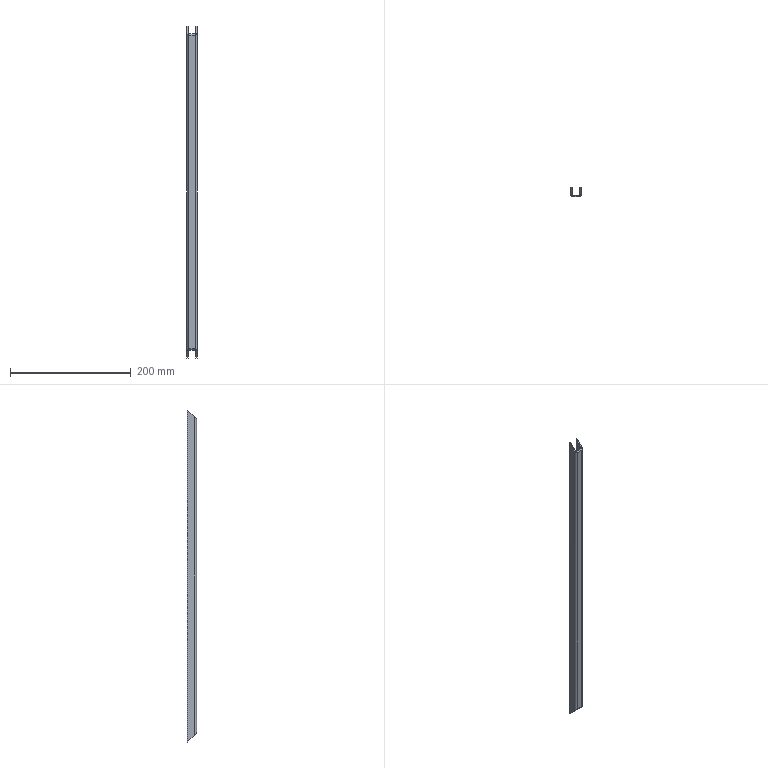Part | STEP file | 1 solid | 14 faces | box 17 x 15 x 549 mm | volume 43355 mm3 | plane 10 | cylinder 4 | commonest cylinder face diameters 3 x2 7 x2
STEP:
#1=CARTESIAN_POINT('',(0.,0.,0.));
#2=DIRECTION('',(0.,0.,1.));
#3=DIRECTION('',(1.,0.,0.));
#4=AXIS2_PLACEMENT_3D('',#1,#2,#3);
#5=CARTESIAN_POINT('',(-6.5,10.,549.));
#6=VERTEX_POINT('',#5);
#7=CARTESIAN_POINT('',(-6.5,10.,0.));
#8=VERTEX_POINT('',#7);
#9=CARTESIAN_POINT('',(-6.5,10.,549.));
#10=DIRECTION('',(0.,0.,-1.));
#11=VECTOR('',#10,1.);
#12=LINE('',#9,#11);
#13=CARTESIAN_POINT('',(-6.5,-5.,549.));
#14=DIRECTION('',(-1.,0.,0.));
#15=DIRECTION('',(0.,0.,1.));
#16=AXIS2_PLACEMENT_3D('',#13,#14,#15);
#17=PLANE('',#16);
#18=CARTESIAN_POINT('',(0.,15.));
#19=DIRECTION('',(-1.,0.));
#20=VECTOR('',#19,1.);
#21=LINE('',#18,#20);
#22=(GEOMETRIC_REPRESENTATION_CONTEXT(2)PARAMETRIC_REPRESENTATION_CONTEXT()REPRESENTATION_CONTEXT('',''));
#23=DEFINITIONAL_REPRESENTATION('',(#21),#22);
#24=PCURVE('',#17,#23);
#25=CARTESIAN_POINT('',(-8.5,10.,549.));
#26=DIRECTION('',(0.,1.,0.));
#27=DIRECTION('',(0.,0.,1.));
#28=AXIS2_PLACEMENT_3D('',#25,#26,#27);
#29=PLANE('',#28);
#30=CARTESIAN_POINT('',(0.,2.));
#31=DIRECTION('',(-1.,0.));
#32=VECTOR('',#31,1.);
#33=LINE('',#30,#32);
#34=(GEOMETRIC_REPRESENTATION_CONTEXT(2)PARAMETRIC_REPRESENTATION_CONTEXT()REPRESENTATION_CONTEXT('',''));
#35=DEFINITIONAL_REPRESENTATION('',(#33),#34);
#36=PCURVE('',#29,#35);
#37=SURFACE_CURVE('',#12,(#24,#36),.PCURVE_S1.);
#38=EDGE_CURVE('',#6,#8,#37,.T.);
#39=ORIENTED_EDGE('',*,*,#38,.F.);
#40=CARTESIAN_POINT('',(-6.5,-1.5,537.5));
#41=VERTEX_POINT('',#40);
#42=CARTESIAN_POINT('',(-6.5,2.5,541.5));
#43=DIRECTION('',(0.,-0.7071,-0.7071));
#44=VECTOR('',#43,1.);
#45=LINE('',#42,#44);
#46=CARTESIAN_POINT('',(-7.5,7.5));
#47=DIRECTION('',(-0.7071,-0.7071));
#48=VECTOR('',#47,1.);
#49=LINE('',#46,#48);
#50=(GEOMETRIC_REPRESENTATION_CONTEXT(2)PARAMETRIC_REPRESENTATION_CONTEXT()REPRESENTATION_CONTEXT('',''));
#51=DEFINITIONAL_REPRESENTATION('',(#49),#50);
#52=PCURVE('',#17,#51);
#53=CARTESIAN_POINT('',(-61.5,10.,549.));
#54=DIRECTION('',(0.,0.7071,-0.7071));
#55=DIRECTION('',(0.,0.7071,0.7071));
#56=AXIS2_PLACEMENT_3D('',#53,#54,#55);
#57=PLANE('',#56);
#58=CARTESIAN_POINT('',(-10.607,55.));
#59=DIRECTION('',(-1.,0.));
#60=VECTOR('',#59,1.);
#61=LINE('',#58,#60);
#62=(GEOMETRIC_REPRESENTATION_CONTEXT(2)PARAMETRIC_REPRESENTATION_CONTEXT()REPRESENTATION_CONTEXT('',''));
#63=DEFINITIONAL_REPRESENTATION('',(#61),#62);
#64=PCURVE('',#57,#63);
#65=SURFACE_CURVE('',#45,(#52,#64),.PCURVE_S1.);
#66=EDGE_CURVE('',#6,#41,#65,.T.);
#67=ORIENTED_EDGE('',*,*,#66,.T.);
#68=CARTESIAN_POINT('',(-6.5,-1.5,11.5));
#69=VERTEX_POINT('',#68);
#70=CARTESIAN_POINT('',(-6.5,-1.5,549.));
#71=DIRECTION('',(0.,0.,-1.));
#72=VECTOR('',#71,1.);
#73=LINE('',#70,#72);
#74=CARTESIAN_POINT('',(0.,3.5));
#75=DIRECTION('',(-1.,0.));
#76=VECTOR('',#75,1.);
#77=LINE('',#74,#76);
#78=(GEOMETRIC_REPRESENTATION_CONTEXT(2)PARAMETRIC_REPRESENTATION_CONTEXT()REPRESENTATION_CONTEXT('',''));
#79=DEFINITIONAL_REPRESENTATION('',(#77),#78);
#80=PCURVE('',#17,#79);
#81=CARTESIAN_POINT('',(-5.,-1.5,549.));
#82=DIRECTION('',(0.,0.,-1.));
#83=DIRECTION('',(-1.,0.,0.));
#84=AXIS2_PLACEMENT_3D('',#81,#82,#83);
#85=CYLINDRICAL_SURFACE('',#84,1.5);
#86=CARTESIAN_POINT('',(6.283,0.));
#87=DIRECTION('',(0.,1.));
#88=VECTOR('',#87,1.);
#89=LINE('',#86,#88);
#90=(GEOMETRIC_REPRESENTATION_CONTEXT(2)PARAMETRIC_REPRESENTATION_CONTEXT()REPRESENTATION_CONTEXT('',''));
#91=DEFINITIONAL_REPRESENTATION('',(#89),#90);
#92=PCURVE('',#85,#91);
#93=SURFACE_CURVE('',#73,(#80,#92),.PCURVE_S1.);
#94=EDGE_CURVE('',#41,#69,#93,.T.);
#95=ORIENTED_EDGE('',*,*,#94,.T.);
#96=CARTESIAN_POINT('',(-6.5,-272.,282.));
#97=DIRECTION('',(0.,0.7071,-0.7071));
#98=VECTOR('',#97,1.);
#99=LINE('',#96,#98);
#100=CARTESIAN_POINT('',(-267.,-267.));
#101=DIRECTION('',(-0.7071,0.7071));
#102=VECTOR('',#101,1.);
#103=LINE('',#100,#102);
#104=(GEOMETRIC_REPRESENTATION_CONTEXT(2)PARAMETRIC_REPRESENTATION_CONTEXT()REPRESENTATION_CONTEXT('',''));
#105=DEFINITIONAL_REPRESENTATION('',(#103),#104);
#106=PCURVE('',#17,#105);
#107=CARTESIAN_POINT('',(-61.5,10.,0.));
#108=DIRECTION('',(0.,0.7071,0.7071));
#109=DIRECTION('',(0.,-0.7071,0.7071));
#110=AXIS2_PLACEMENT_3D('',#107,#108,#109);
#111=PLANE('',#110);
#112=CARTESIAN_POINT('',(398.808,55.));
#113=DIRECTION('',(-1.,0.));
#114=VECTOR('',#113,1.);
#115=LINE('',#112,#114);
#116=(GEOMETRIC_REPRESENTATION_CONTEXT(2)PARAMETRIC_REPRESENTATION_CONTEXT()REPRESENTATION_CONTEXT('',''));
#117=DEFINITIONAL_REPRESENTATION('',(#115),#116);
#118=PCURVE('',#111,#117);
#119=SURFACE_CURVE('',#99,(#106,#118),.PCURVE_S1.);
#120=EDGE_CURVE('',#69,#8,#119,.T.);
#121=ORIENTED_EDGE('',*,*,#120,.T.);
#122=EDGE_LOOP('',(#39,#67,#95,#121));
#123=FACE_BOUND('',#122,.T.);
#124=ADVANCED_FACE('',(#123),#17,.F.);
#125=CARTESIAN_POINT('',(-8.5,10.,0.));
#126=VERTEX_POINT('',#125);
#127=CARTESIAN_POINT('',(-8.5,10.,0.));
#128=DIRECTION('',(1.,0.,0.));
#129=VECTOR('',#128,1.);
#130=LINE('',#127,#129);
#131=CARTESIAN_POINT('',(-549.,0.));
#132=DIRECTION('',(0.,1.));
#133=VECTOR('',#132,1.);
#134=LINE('',#131,#133);
#135=(GEOMETRIC_REPRESENTATION_CONTEXT(2)PARAMETRIC_REPRESENTATION_CONTEXT()REPRESENTATION_CONTEXT('',''));
#136=DEFINITIONAL_REPRESENTATION('',(#134),#135);
#137=PCURVE('',#29,#136);
#138=CARTESIAN_POINT('',(0.,53.));
#139=DIRECTION('',(0.,1.));
#140=VECTOR('',#139,1.);
#141=LINE('',#138,#140);
#142=(GEOMETRIC_REPRESENTATION_CONTEXT(2)PARAMETRIC_REPRESENTATION_CONTEXT()REPRESENTATION_CONTEXT('',''));
#143=DEFINITIONAL_REPRESENTATION('',(#141),#142);
#144=PCURVE('',#111,#143);
#145=SURFACE_CURVE('',#130,(#137,#144),.PCURVE_S1.);
#146=EDGE_CURVE('',#126,#8,#145,.T.);
#147=ORIENTED_EDGE('',*,*,#146,.F.);
#148=CARTESIAN_POINT('',(-8.5,10.,549.));
#149=VERTEX_POINT('',#148);
#150=CARTESIAN_POINT('',(-8.5,10.,549.));
#151=DIRECTION('',(0.,0.,-1.));
#152=VECTOR('',#151,1.);
#153=LINE('',#150,#152);
#154=CARTESIAN_POINT('',(0.,0.));
#155=DIRECTION('',(-1.,0.));
#156=VECTOR('',#155,1.);
#157=LINE('',#154,#156);
#158=(GEOMETRIC_REPRESENTATION_CONTEXT(2)PARAMETRIC_REPRESENTATION_CONTEXT()REPRESENTATION_CONTEXT('',''));
#159=DEFINITIONAL_REPRESENTATION('',(#157),#158);
#160=PCURVE('',#29,#159);
#161=CARTESIAN_POINT('',(-8.5,-5.,549.));
#162=DIRECTION('',(-1.,0.,0.));
#163=DIRECTION('',(0.,0.,1.));
#164=AXIS2_PLACEMENT_3D('',#161,#162,#163);
#165=PLANE('',#164);
#166=CARTESIAN_POINT('',(0.,15.));
#167=DIRECTION('',(-1.,0.));
#168=VECTOR('',#167,1.);
#169=LINE('',#166,#168);
#170=(GEOMETRIC_REPRESENTATION_CONTEXT(2)PARAMETRIC_REPRESENTATION_CONTEXT()REPRESENTATION_CONTEXT('',''));
#171=DEFINITIONAL_REPRESENTATION('',(#169),#170);
#172=PCURVE('',#165,#171);
#173=SURFACE_CURVE('',#153,(#160,#172),.PCURVE_S1.);
#174=EDGE_CURVE('',#149,#126,#173,.T.);
#175=ORIENTED_EDGE('',*,*,#174,.F.);
#176=CARTESIAN_POINT('',(-8.5,10.,549.));
#177=DIRECTION('',(1.,0.,0.));
#178=VECTOR('',#177,1.);
#179=LINE('',#176,#178);
#180=CARTESIAN_POINT('',(0.,0.));
#181=DIRECTION('',(0.,1.));
#182=VECTOR('',#181,1.);
#183=LINE('',#180,#182);
#184=(GEOMETRIC_REPRESENTATION_CONTEXT(2)PARAMETRIC_REPRESENTATION_CONTEXT()REPRESENTATION_CONTEXT('',''));
#185=DEFINITIONAL_REPRESENTATION('',(#183),#184);
#186=PCURVE('',#29,#185);
#187=CARTESIAN_POINT('',(0.,53.));
#188=DIRECTION('',(0.,1.));
#189=VECTOR('',#188,1.);
#190=LINE('',#187,#189);
#191=(GEOMETRIC_REPRESENTATION_CONTEXT(2)PARAMETRIC_REPRESENTATION_CONTEXT()REPRESENTATION_CONTEXT('',''));
#192=DEFINITIONAL_REPRESENTATION('',(#190),#191);
#193=PCURVE('',#57,#192);
#194=SURFACE_CURVE('',#179,(#186,#193),.PCURVE_S1.);
#195=EDGE_CURVE('',#149,#6,#194,.T.);
#196=ORIENTED_EDGE('',*,*,#195,.T.);
#197=ORIENTED_EDGE('',*,*,#38,.T.);
#198=EDGE_LOOP('',(#147,#175,#196,#197));
#199=FACE_BOUND('',#198,.T.);
#200=ADVANCED_FACE('',(#199),#29,.T.);
#201=CARTESIAN_POINT('',(-8.5,-1.5,537.5));
#202=VERTEX_POINT('',#201);
#203=CARTESIAN_POINT('',(-8.5,2.5,541.5));
#204=DIRECTION('',(0.,-0.7071,-0.7071));
#205=VECTOR('',#204,1.);
#206=LINE('',#203,#205);
#207=CARTESIAN_POINT('',(-7.5,7.5));
#208=DIRECTION('',(-0.7071,-0.7071));
#209=VECTOR('',#208,1.);
#210=LINE('',#207,#209);
#211=(GEOMETRIC_REPRESENTATION_CONTEXT(2)PARAMETRIC_REPRESENTATION_CONTEXT()REPRESENTATION_CONTEXT('',''));
#212=DEFINITIONAL_REPRESENTATION('',(#210),#211);
#213=PCURVE('',#165,#212);
#214=CARTESIAN_POINT('',(-10.607,53.));
#215=DIRECTION('',(-1.,0.));
#216=VECTOR('',#215,1.);
#217=LINE('',#214,#216);
#218=(GEOMETRIC_REPRESENTATION_CONTEXT(2)PARAMETRIC_REPRESENTATION_CONTEXT()REPRESENTATION_CONTEXT('',''));
#219=DEFINITIONAL_REPRESENTATION('',(#217),#218);
#220=PCURVE('',#57,#219);
#221=SURFACE_CURVE('',#206,(#213,#220),.PCURVE_S1.);
#222=EDGE_CURVE('',#149,#202,#221,.T.);
#223=ORIENTED_EDGE('',*,*,#222,.F.);
#224=ORIENTED_EDGE('',*,*,#174,.T.);
#225=CARTESIAN_POINT('',(-8.5,-1.5,11.5));
#226=VERTEX_POINT('',#225);
#227=CARTESIAN_POINT('',(-8.5,-272.,282.));
#228=DIRECTION('',(0.,0.7071,-0.7071));
#229=VECTOR('',#228,1.);
#230=LINE('',#227,#229);
#231=CARTESIAN_POINT('',(-267.,-267.));
#232=DIRECTION('',(-0.7071,0.7071));
#233=VECTOR('',#232,1.);
#234=LINE('',#231,#233);
#235=(GEOMETRIC_REPRESENTATION_CONTEXT(2)PARAMETRIC_REPRESENTATION_CONTEXT()REPRESENTATION_CONTEXT('',''));
#236=DEFINITIONAL_REPRESENTATION('',(#234),#235);
#237=PCURVE('',#165,#236);
#238=CARTESIAN_POINT('',(398.808,53.));
#239=DIRECTION('',(-1.,0.));
#240=VECTOR('',#239,1.);
#241=LINE('',#238,#240);
#242=(GEOMETRIC_REPRESENTATION_CONTEXT(2)PARAMETRIC_REPRESENTATION_CONTEXT()REPRESENTATION_CONTEXT('',''));
#243=DEFINITIONAL_REPRESENTATION('',(#241),#242);
#244=PCURVE('',#111,#243);
#245=SURFACE_CURVE('',#230,(#237,#244),.PCURVE_S1.);
#246=EDGE_CURVE('',#226,#126,#245,.T.);
#247=ORIENTED_EDGE('',*,*,#246,.F.);
#248=CARTESIAN_POINT('',(-8.5,-1.5,549.));
#249=DIRECTION('',(0.,0.,-1.));
#250=VECTOR('',#249,1.);
#251=LINE('',#248,#250);
#252=CARTESIAN_POINT('',(0.,3.5));
#253=DIRECTION('',(-1.,0.));
#254=VECTOR('',#253,1.);
#255=LINE('',#252,#254);
#256=(GEOMETRIC_REPRESENTATION_CONTEXT(2)PARAMETRIC_REPRESENTATION_CONTEXT()REPRESENTATION_CONTEXT('',''));
#257=DEFINITIONAL_REPRESENTATION('',(#255),#256);
#258=PCURVE('',#165,#257);
#259=CARTESIAN_POINT('',(-5.,-1.5,549.));
#260=DIRECTION('',(0.,0.,-1.));
#261=DIRECTION('',(-1.,0.,0.));
#262=AXIS2_PLACEMENT_3D('',#259,#260,#261);
#263=CYLINDRICAL_SURFACE('',#262,3.5);
#264=CARTESIAN_POINT('',(6.283,0.));
#265=DIRECTION('',(0.,1.));
#266=VECTOR('',#265,1.);
#267=LINE('',#264,#266);
#268=(GEOMETRIC_REPRESENTATION_CONTEXT(2)PARAMETRIC_REPRESENTATION_CONTEXT()REPRESENTATION_CONTEXT('',''));
#269=DEFINITIONAL_REPRESENTATION('',(#267),#268);
#270=PCURVE('',#263,#269);
#271=SURFACE_CURVE('',#251,(#258,#270),.PCURVE_S1.);
#272=EDGE_CURVE('',#202,#226,#271,.T.);
#273=ORIENTED_EDGE('',*,*,#272,.F.);
#274=EDGE_LOOP('',(#223,#224,#247,#273));
#275=FACE_BOUND('',#274,.T.);
#276=ADVANCED_FACE('',(#275),#165,.T.);
#277=CARTESIAN_POINT('',(-5.,-5.,534.));
#278=VERTEX_POINT('',#277);
#279=CARTESIAN_POINT('',(-8.5,-1.5,537.5));
#280=CARTESIAN_POINT('',(-8.5,-3.55,535.45));
#281=CARTESIAN_POINT('',(-7.05,-5.,534.));
#282=CARTESIAN_POINT('',(-5.,-5.,534.));
#283=(BOUNDED_CURVE()B_SPLINE_CURVE(3,(#279,#280,#281,#282),.UNSPECIFIED.,.F.,.F.)B_SPLINE_CURVE_WITH_KNOTS((4,4),(4.712,6.283),.PIECEWISE_BEZIER_KNOTS.)CURVE()GEOMETRIC_REPRESENTATION_ITEM()RATIONAL_B_SPLINE_CURVE((1.,0.8047,0.8047,1.))REPRESENTATION_ITEM(''));
#284=CARTESIAN_POINT('',(6.283,11.5));
#285=CARTESIAN_POINT('',(6.262,11.575));
#286=CARTESIAN_POINT('',(6.218,11.727));
#287=CARTESIAN_POINT('',(6.152,11.96));
#288=CARTESIAN_POINT('',(6.083,12.196));
#289=CARTESIAN_POINT('',(6.013,12.433));
#290=CARTESIAN_POINT('',(5.942,12.671));
#291=CARTESIAN_POINT('',(5.87,12.906));
#292=CARTESIAN_POINT('',(5.797,13.137));
#293=CARTESIAN_POINT('',(5.723,13.362));
#294=CARTESIAN_POINT('',(5.648,13.578));
#295=CARTESIAN_POINT('',(5.573,13.784));
#296=CARTESIAN_POINT('',(5.498,13.977));
#297=CARTESIAN_POINT('',(5.422,14.157));
#298=CARTESIAN_POINT('',(5.347,14.32));
#299=CARTESIAN_POINT('',(5.273,14.468));
#300=CARTESIAN_POINT('',(5.199,14.597));
#301=CARTESIAN_POINT('',(5.125,14.709));
#302=CARTESIAN_POINT('',(5.053,14.802));
#303=CARTESIAN_POINT('',(4.982,14.876));
#304=CARTESIAN_POINT('',(4.912,14.933));
#305=CARTESIAN_POINT('',(4.844,14.972));
#306=CARTESIAN_POINT('',(4.777,14.995));
#307=CARTESIAN_POINT('',(4.734,15.));
#308=CARTESIAN_POINT('',(4.712,15.));
#309=B_SPLINE_CURVE_WITH_KNOTS('',3,(#284,#285,#286,#287,#288,#289,#290,#291,#292,#293,#294,#295,#296,#297,#298,#299,#300,#301,#302,#303,#304,#305,#306,#307,#308),.UNSPECIFIED.,.F.,.F.,(4,1,1,1,1,1,1,1,1,1,1,1,1,1,1,1,1,1,1,1,1,1,4),(4.712,4.784,4.855,4.927,4.998,5.069,5.141,5.212,5.284,5.355,5.426,5.498,5.569,5.641,5.712,5.783,5.855,5.926,5.998,6.069,6.14,6.212,6.283),.QUASI_UNIFORM_KNOTS.);
#310=(GEOMETRIC_REPRESENTATION_CONTEXT(2)PARAMETRIC_REPRESENTATION_CONTEXT()REPRESENTATION_CONTEXT('',''));
#311=DEFINITIONAL_REPRESENTATION('',(#309),#310);
#312=PCURVE('',#263,#311);
#313=CARTESIAN_POINT('',(-16.263,53.));
#314=CARTESIAN_POINT('',(-19.163,53.));
#315=CARTESIAN_POINT('',(-21.213,54.45));
#316=CARTESIAN_POINT('',(-21.213,56.5));
#317=(BOUNDED_CURVE()B_SPLINE_CURVE(3,(#313,#314,#315,#316),.UNSPECIFIED.,.F.,.F.)B_SPLINE_CURVE_WITH_KNOTS((4,4),(4.712,6.283),.PIECEWISE_BEZIER_KNOTS.)CURVE()GEOMETRIC_REPRESENTATION_ITEM()RATIONAL_B_SPLINE_CURVE((1.,0.8047,0.8047,1.))REPRESENTATION_ITEM(''));
#318=(GEOMETRIC_REPRESENTATION_CONTEXT(2)PARAMETRIC_REPRESENTATION_CONTEXT()REPRESENTATION_CONTEXT('',''));
#319=DEFINITIONAL_REPRESENTATION('',(#317),#318);
#320=PCURVE('',#57,#319);
#321=SURFACE_CURVE('',#283,(#312,#320),.PCURVE_S1.);
#322=EDGE_CURVE('',#202,#278,#321,.T.);
#323=ORIENTED_EDGE('',*,*,#322,.F.);
#324=ORIENTED_EDGE('',*,*,#272,.T.);
#325=CARTESIAN_POINT('',(-5.,-5.,15.));
#326=VERTEX_POINT('',#325);
#327=CARTESIAN_POINT('',(-5.,-5.,15.));
#328=CARTESIAN_POINT('',(-7.05,-5.,15.));
#329=CARTESIAN_POINT('',(-8.5,-3.55,13.55));
#330=CARTESIAN_POINT('',(-8.5,-1.5,11.5));
#331=(BOUNDED_CURVE()B_SPLINE_CURVE(3,(#327,#328,#329,#330),.UNSPECIFIED.,.F.,.F.)B_SPLINE_CURVE_WITH_KNOTS((4,4),(3.142,4.712),.PIECEWISE_BEZIER_KNOTS.)CURVE()GEOMETRIC_REPRESENTATION_ITEM()RATIONAL_B_SPLINE_CURVE((1.,0.8047,0.8047,1.))REPRESENTATION_ITEM(''));
#332=CARTESIAN_POINT('',(4.712,534.));
#333=CARTESIAN_POINT('',(4.734,534.));
#334=CARTESIAN_POINT('',(4.777,534.005));
#335=CARTESIAN_POINT('',(4.844,534.028));
#336=CARTESIAN_POINT('',(4.912,534.067));
#337=CARTESIAN_POINT('',(4.982,534.124));
#338=CARTESIAN_POINT('',(5.053,534.198));
#339=CARTESIAN_POINT('',(5.125,534.291));
#340=CARTESIAN_POINT('',(5.199,534.403));
#341=CARTESIAN_POINT('',(5.273,534.532));
#342=CARTESIAN_POINT('',(5.347,534.68));
#343=CARTESIAN_POINT('',(5.422,534.843));
#344=CARTESIAN_POINT('',(5.498,535.023));
#345=CARTESIAN_POINT('',(5.573,535.216));
#346=CARTESIAN_POINT('',(5.648,535.422));
#347=CARTESIAN_POINT('',(5.723,535.638));
#348=CARTESIAN_POINT('',(5.797,535.863));
#349=CARTESIAN_POINT('',(5.87,536.094));
#350=CARTESIAN_POINT('',(5.942,536.329));
#351=CARTESIAN_POINT('',(6.013,536.567));
#352=CARTESIAN_POINT('',(6.083,536.804));
#353=CARTESIAN_POINT('',(6.152,537.04));
#354=CARTESIAN_POINT('',(6.218,537.273));
#355=CARTESIAN_POINT('',(6.262,537.425));
#356=CARTESIAN_POINT('',(6.283,537.5));
#357=B_SPLINE_CURVE_WITH_KNOTS('',3,(#332,#333,#334,#335,#336,#337,#338,#339,#340,#341,#342,#343,#344,#345,#346,#347,#348,#349,#350,#351,#352,#353,#354,#355,#356),.UNSPECIFIED.,.F.,.F.,(4,1,1,1,1,1,1,1,1,1,1,1,1,1,1,1,1,1,1,1,1,1,4),(3.142,3.213,3.284,3.356,3.427,3.499,3.57,3.641,3.713,3.784,3.856,3.927,3.998,4.07,4.141,4.213,4.284,4.355,4.427,4.498,4.57,4.641,4.712),.QUASI_UNIFORM_KNOTS.);
#358=(GEOMETRIC_REPRESENTATION_CONTEXT(2)PARAMETRIC_REPRESENTATION_CONTEXT()REPRESENTATION_CONTEXT('',''));
#359=DEFINITIONAL_REPRESENTATION('',(#357),#358);
#360=PCURVE('',#263,#359);
#361=CARTESIAN_POINT('',(21.213,56.5));
#362=CARTESIAN_POINT('',(21.213,54.45));
#363=CARTESIAN_POINT('',(19.163,53.));
#364=CARTESIAN_POINT('',(16.263,53.));
#365=(BOUNDED_CURVE()B_SPLINE_CURVE(3,(#361,#362,#363,#364),.UNSPECIFIED.,.F.,.F.)B_SPLINE_CURVE_WITH_KNOTS((4,4),(3.142,4.712),.PIECEWISE_BEZIER_KNOTS.)CURVE()GEOMETRIC_REPRESENTATION_ITEM()RATIONAL_B_SPLINE_CURVE((1.,0.8047,0.8047,1.))REPRESENTATION_ITEM(''));
#366=(GEOMETRIC_REPRESENTATION_CONTEXT(2)PARAMETRIC_REPRESENTATION_CONTEXT()REPRESENTATION_CONTEXT('',''));
#367=DEFINITIONAL_REPRESENTATION('',(#365),#366);
#368=PCURVE('',#111,#367);
#369=SURFACE_CURVE('',#331,(#360,#368),.PCURVE_S1.);
#370=EDGE_CURVE('',#326,#226,#369,.T.);
#371=ORIENTED_EDGE('',*,*,#370,.F.);
#372=CARTESIAN_POINT('',(-5.,-5.,549.));
#373=DIRECTION('',(0.,0.,-1.));
#374=VECTOR('',#373,1.);
#375=LINE('',#372,#374);
#376=CARTESIAN_POINT('',(4.712,0.));
#377=DIRECTION('',(0.,1.));
#378=VECTOR('',#377,1.);
#379=LINE('',#376,#378);
#380=(GEOMETRIC_REPRESENTATION_CONTEXT(2)PARAMETRIC_REPRESENTATION_CONTEXT()REPRESENTATION_CONTEXT('',''));
#381=DEFINITIONAL_REPRESENTATION('',(#379),#380);
#382=PCURVE('',#263,#381);
#383=CARTESIAN_POINT('',(-8.5,-5.,549.));
#384=DIRECTION('',(0.,-1.,0.));
#385=DIRECTION('',(0.,0.,-1.));
#386=AXIS2_PLACEMENT_3D('',#383,#384,#385);
#387=PLANE('',#386);
#388=CARTESIAN_POINT('',(0.,3.5));
#389=DIRECTION('',(1.,0.));
#390=VECTOR('',#389,1.);
#391=LINE('',#388,#390);
#392=(GEOMETRIC_REPRESENTATION_CONTEXT(2)PARAMETRIC_REPRESENTATION_CONTEXT()REPRESENTATION_CONTEXT('',''));
#393=DEFINITIONAL_REPRESENTATION('',(#391),#392);
#394=PCURVE('',#387,#393);
#395=SURFACE_CURVE('',#375,(#382,#394),.PCURVE_S1.);
#396=EDGE_CURVE('',#278,#326,#395,.T.);
#397=ORIENTED_EDGE('',*,*,#396,.F.);
#398=EDGE_LOOP('',(#323,#324,#371,#397));
#399=FACE_BOUND('',#398,.T.);
#400=ADVANCED_FACE('',(#399),#263,.T.);
#401=CARTESIAN_POINT('',(5.,-5.,534.));
#402=VERTEX_POINT('',#401);
#403=CARTESIAN_POINT('',(-61.5,-5.,534.));
#404=DIRECTION('',(1.,0.,0.));
#405=VECTOR('',#404,1.);
#406=LINE('',#403,#405);
#407=CARTESIAN_POINT('',(15.,-53.));
#408=DIRECTION('',(0.,1.));
#409=VECTOR('',#408,1.);
#410=LINE('',#407,#409);
#411=(GEOMETRIC_REPRESENTATION_CONTEXT(2)PARAMETRIC_REPRESENTATION_CONTEXT()REPRESENTATION_CONTEXT('',''));
#412=DEFINITIONAL_REPRESENTATION('',(#410),#411);
#413=PCURVE('',#387,#412);
#414=CARTESIAN_POINT('',(-21.213,0.));
#415=DIRECTION('',(0.,1.));
#416=VECTOR('',#415,1.);
#417=LINE('',#414,#416);
#418=(GEOMETRIC_REPRESENTATION_CONTEXT(2)PARAMETRIC_REPRESENTATION_CONTEXT()REPRESENTATION_CONTEXT('',''));
#419=DEFINITIONAL_REPRESENTATION('',(#417),#418);
#420=PCURVE('',#57,#419);
#421=SURFACE_CURVE('',#406,(#413,#420),.PCURVE_S1.);
#422=EDGE_CURVE('',#278,#402,#421,.T.);
#423=ORIENTED_EDGE('',*,*,#422,.F.);
#424=ORIENTED_EDGE('',*,*,#396,.T.);
#425=CARTESIAN_POINT('',(5.,-5.,15.));
#426=VERTEX_POINT('',#425);
#427=CARTESIAN_POINT('',(-61.5,-5.,15.));
#428=DIRECTION('',(1.,0.,0.));
#429=VECTOR('',#428,1.);
#430=LINE('',#427,#429);
#431=CARTESIAN_POINT('',(534.,-53.));
#432=DIRECTION('',(0.,1.));
#433=VECTOR('',#432,1.);
#434=LINE('',#431,#433);
#435=(GEOMETRIC_REPRESENTATION_CONTEXT(2)PARAMETRIC_REPRESENTATION_CONTEXT()REPRESENTATION_CONTEXT('',''));
#436=DEFINITIONAL_REPRESENTATION('',(#434),#435);
#437=PCURVE('',#387,#436);
#438=CARTESIAN_POINT('',(21.213,0.));
#439=DIRECTION('',(0.,1.));
#440=VECTOR('',#439,1.);
#441=LINE('',#438,#440);
#442=(GEOMETRIC_REPRESENTATION_CONTEXT(2)PARAMETRIC_REPRESENTATION_CONTEXT()REPRESENTATION_CONTEXT('',''));
#443=DEFINITIONAL_REPRESENTATION('',(#441),#442);
#444=PCURVE('',#111,#443);
#445=SURFACE_CURVE('',#430,(#437,#444),.PCURVE_S1.);
#446=EDGE_CURVE('',#326,#426,#445,.T.);
#447=ORIENTED_EDGE('',*,*,#446,.T.);
#448=CARTESIAN_POINT('',(5.,-5.,549.));
#449=DIRECTION('',(0.,0.,-1.));
#450=VECTOR('',#449,1.);
#451=LINE('',#448,#450);
#452=CARTESIAN_POINT('',(0.,13.5));
#453=DIRECTION('',(1.,0.));
#454=VECTOR('',#453,1.);
#455=LINE('',#452,#454);
#456=(GEOMETRIC_REPRESENTATION_CONTEXT(2)PARAMETRIC_REPRESENTATION_CONTEXT()REPRESENTATION_CONTEXT('',''));
#457=DEFINITIONAL_REPRESENTATION('',(#455),#456);
#458=PCURVE('',#387,#457);
#459=CARTESIAN_POINT('',(5.,-1.5,549.));
#460=DIRECTION('',(0.,0.,-1.));
#461=DIRECTION('',(-1.,0.,0.));
#462=AXIS2_PLACEMENT_3D('',#459,#460,#461);
#463=CYLINDRICAL_SURFACE('',#462,3.5);
#464=CARTESIAN_POINT('',(4.712,0.));
#465=DIRECTION('',(0.,1.));
#466=VECTOR('',#465,1.);
#467=LINE('',#464,#466);
#468=(GEOMETRIC_REPRESENTATION_CONTEXT(2)PARAMETRIC_REPRESENTATION_CONTEXT()REPRESENTATION_CONTEXT('',''));
#469=DEFINITIONAL_REPRESENTATION('',(#467),#468);
#470=PCURVE('',#463,#469);
#471=SURFACE_CURVE('',#451,(#458,#470),.PCURVE_S1.);
#472=EDGE_CURVE('',#402,#426,#471,.T.);
#473=ORIENTED_EDGE('',*,*,#472,.F.);
#474=EDGE_LOOP('',(#423,#424,#447,#473));
#475=FACE_BOUND('',#474,.T.);
#476=ADVANCED_FACE('',(#475),#387,.T.);
#477=CARTESIAN_POINT('',(8.5,-1.5,537.5));
#478=VERTEX_POINT('',#477);
#479=CARTESIAN_POINT('',(5.,-5.,534.));
#480=CARTESIAN_POINT('',(7.05,-5.,534.));
#481=CARTESIAN_POINT('',(8.5,-3.55,535.45));
#482=CARTESIAN_POINT('',(8.5,-1.5,537.5));
#483=(BOUNDED_CURVE()B_SPLINE_CURVE(3,(#479,#480,#481,#482),.UNSPECIFIED.,.F.,.F.)B_SPLINE_CURVE_WITH_KNOTS((4,4),(0.,1.571),.PIECEWISE_BEZIER_KNOTS.)CURVE()GEOMETRIC_REPRESENTATION_ITEM()RATIONAL_B_SPLINE_CURVE((1.,0.8047,0.8047,1.))REPRESENTATION_ITEM(''));
#484=CARTESIAN_POINT('',(4.712,15.));
#485=CARTESIAN_POINT('',(4.691,15.));
#486=CARTESIAN_POINT('',(4.648,14.995));
#487=CARTESIAN_POINT('',(4.581,14.972));
#488=CARTESIAN_POINT('',(4.512,14.933));
#489=CARTESIAN_POINT('',(4.443,14.876));
#490=CARTESIAN_POINT('',(4.372,14.802));
#491=CARTESIAN_POINT('',(4.299,14.709));
#492=CARTESIAN_POINT('',(4.226,14.597));
#493=CARTESIAN_POINT('',(4.152,14.468));
#494=CARTESIAN_POINT('',(4.077,14.32));
#495=CARTESIAN_POINT('',(4.002,14.157));
#496=CARTESIAN_POINT('',(3.927,13.977));
#497=CARTESIAN_POINT('',(3.852,13.784));
#498=CARTESIAN_POINT('',(3.777,13.578));
#499=CARTESIAN_POINT('',(3.702,13.362));
#500=CARTESIAN_POINT('',(3.628,13.137));
#501=CARTESIAN_POINT('',(3.555,12.906));
#502=CARTESIAN_POINT('',(3.482,12.671));
#503=CARTESIAN_POINT('',(3.411,12.433));
#504=CARTESIAN_POINT('',(3.342,12.196));
#505=CARTESIAN_POINT('',(3.273,11.96));
#506=CARTESIAN_POINT('',(3.206,11.727));
#507=CARTESIAN_POINT('',(3.163,11.575));
#508=CARTESIAN_POINT('',(3.142,11.5));
#509=B_SPLINE_CURVE_WITH_KNOTS('',3,(#484,#485,#486,#487,#488,#489,#490,#491,#492,#493,#494,#495,#496,#497,#498,#499,#500,#501,#502,#503,#504,#505,#506,#507,#508),.UNSPECIFIED.,.F.,.F.,(4,1,1,1,1,1,1,1,1,1,1,1,1,1,1,1,1,1,1,1,1,1,4),(0.,0.0714,0.1428,0.2142,0.2856,0.357,0.4284,0.4998,0.5712,0.6426,0.714,0.7854,0.8568,0.9282,0.9996,1.071,1.142,1.214,1.285,1.357,1.428,1.499,1.571),.QUASI_UNIFORM_KNOTS.);
#510=(GEOMETRIC_REPRESENTATION_CONTEXT(2)PARAMETRIC_REPRESENTATION_CONTEXT()REPRESENTATION_CONTEXT('',''));
#511=DEFINITIONAL_REPRESENTATION('',(#509),#510);
#512=PCURVE('',#463,#511);
#513=CARTESIAN_POINT('',(-21.213,66.5));
#514=CARTESIAN_POINT('',(-21.213,68.55));
#515=CARTESIAN_POINT('',(-19.163,70.));
#516=CARTESIAN_POINT('',(-16.263,70.));
#517=(BOUNDED_CURVE()B_SPLINE_CURVE(3,(#513,#514,#515,#516),.UNSPECIFIED.,.F.,.F.)B_SPLINE_CURVE_WITH_KNOTS((4,4),(0.,1.571),.PIECEWISE_BEZIER_KNOTS.)CURVE()GEOMETRIC_REPRESENTATION_ITEM()RATIONAL_B_SPLINE_CURVE((1.,0.8047,0.8047,1.))REPRESENTATION_ITEM(''));
#518=(GEOMETRIC_REPRESENTATION_CONTEXT(2)PARAMETRIC_REPRESENTATION_CONTEXT()REPRESENTATION_CONTEXT('',''));
#519=DEFINITIONAL_REPRESENTATION('',(#517),#518);
#520=PCURVE('',#57,#519);
#521=SURFACE_CURVE('',#483,(#512,#520),.PCURVE_S1.);
#522=EDGE_CURVE('',#402,#478,#521,.T.);
#523=ORIENTED_EDGE('',*,*,#522,.F.);
#524=ORIENTED_EDGE('',*,*,#472,.T.);
#525=CARTESIAN_POINT('',(8.5,-1.5,11.5));
#526=VERTEX_POINT('',#525);
#527=CARTESIAN_POINT('',(8.5,-1.5,11.5));
#528=CARTESIAN_POINT('',(8.5,-3.55,13.55));
#529=CARTESIAN_POINT('',(7.05,-5.,15.));
#530=CARTESIAN_POINT('',(5.,-5.,15.));
#531=(BOUNDED_CURVE()B_SPLINE_CURVE(3,(#527,#528,#529,#530),.UNSPECIFIED.,.F.,.F.)B_SPLINE_CURVE_WITH_KNOTS((4,4),(1.571,3.142),.PIECEWISE_BEZIER_KNOTS.)CURVE()GEOMETRIC_REPRESENTATION_ITEM()RATIONAL_B_SPLINE_CURVE((1.,0.8047,0.8047,1.))REPRESENTATION_ITEM(''));
#532=CARTESIAN_POINT('',(3.142,537.5));
#533=CARTESIAN_POINT('',(3.163,537.425));
#534=CARTESIAN_POINT('',(3.206,537.273));
#535=CARTESIAN_POINT('',(3.273,537.04));
#536=CARTESIAN_POINT('',(3.342,536.804));
#537=CARTESIAN_POINT('',(3.411,536.567));
#538=CARTESIAN_POINT('',(3.482,536.329));
#539=CARTESIAN_POINT('',(3.555,536.094));
#540=CARTESIAN_POINT('',(3.628,535.863));
#541=CARTESIAN_POINT('',(3.702,535.638));
#542=CARTESIAN_POINT('',(3.777,535.422));
#543=CARTESIAN_POINT('',(3.852,535.216));
#544=CARTESIAN_POINT('',(3.927,535.023));
#545=CARTESIAN_POINT('',(4.002,534.843));
#546=CARTESIAN_POINT('',(4.077,534.68));
#547=CARTESIAN_POINT('',(4.152,534.532));
#548=CARTESIAN_POINT('',(4.226,534.403));
#549=CARTESIAN_POINT('',(4.299,534.291));
#550=CARTESIAN_POINT('',(4.372,534.198));
#551=CARTESIAN_POINT('',(4.443,534.124));
#552=CARTESIAN_POINT('',(4.512,534.067));
#553=CARTESIAN_POINT('',(4.581,534.028));
#554=CARTESIAN_POINT('',(4.648,534.005));
#555=CARTESIAN_POINT('',(4.691,534.));
#556=CARTESIAN_POINT('',(4.712,534.));
#557=B_SPLINE_CURVE_WITH_KNOTS('',3,(#532,#533,#534,#535,#536,#537,#538,#539,#540,#541,#542,#543,#544,#545,#546,#547,#548,#549,#550,#551,#552,#553,#554,#555,#556),.UNSPECIFIED.,.F.,.F.,(4,1,1,1,1,1,1,1,1,1,1,1,1,1,1,1,1,1,1,1,1,1,4),(1.571,1.642,1.714,1.785,1.856,1.928,1.999,2.071,2.142,2.213,2.285,2.356,2.428,2.499,2.57,2.642,2.713,2.785,2.856,2.927,2.999,3.07,3.142),.QUASI_UNIFORM_KNOTS.);
#558=(GEOMETRIC_REPRESENTATION_CONTEXT(2)PARAMETRIC_REPRESENTATION_CONTEXT()REPRESENTATION_CONTEXT('',''));
#559=DEFINITIONAL_REPRESENTATION('',(#557),#558);
#560=PCURVE('',#463,#559);
#561=CARTESIAN_POINT('',(16.263,70.));
#562=CARTESIAN_POINT('',(19.163,70.));
#563=CARTESIAN_POINT('',(21.213,68.55));
#564=CARTESIAN_POINT('',(21.213,66.5));
#565=(BOUNDED_CURVE()B_SPLINE_CURVE(3,(#561,#562,#563,#564),.UNSPECIFIED.,.F.,.F.)B_SPLINE_CURVE_WITH_KNOTS((4,4),(1.571,3.142),.PIECEWISE_BEZIER_KNOTS.)CURVE()GEOMETRIC_REPRESENTATION_ITEM()RATIONAL_B_SPLINE_CURVE((1.,0.8047,0.8047,1.))REPRESENTATION_ITEM(''));
#566=(GEOMETRIC_REPRESENTATION_CONTEXT(2)PARAMETRIC_REPRESENTATION_CONTEXT()REPRESENTATION_CONTEXT('',''));
#567=DEFINITIONAL_REPRESENTATION('',(#565),#566);
#568=PCURVE('',#111,#567);
#569=SURFACE_CURVE('',#531,(#560,#568),.PCURVE_S1.);
#570=EDGE_CURVE('',#526,#426,#569,.T.);
#571=ORIENTED_EDGE('',*,*,#570,.F.);
#572=CARTESIAN_POINT('',(8.5,-1.5,549.));
#573=DIRECTION('',(0.,0.,-1.));
#574=VECTOR('',#573,1.);
#575=LINE('',#572,#574);
#576=CARTESIAN_POINT('',(3.142,0.));
#577=DIRECTION('',(0.,1.));
#578=VECTOR('',#577,1.);
#579=LINE('',#576,#578);
#580=(GEOMETRIC_REPRESENTATION_CONTEXT(2)PARAMETRIC_REPRESENTATION_CONTEXT()REPRESENTATION_CONTEXT('',''));
#581=DEFINITIONAL_REPRESENTATION('',(#579),#580);
#582=PCURVE('',#463,#581);
#583=CARTESIAN_POINT('',(8.5,-5.,549.));
#584=DIRECTION('',(1.,0.,0.));
#585=DIRECTION('',(0.,0.,-1.));
#586=AXIS2_PLACEMENT_3D('',#583,#584,#585);
#587=PLANE('',#586);
#588=CARTESIAN_POINT('',(0.,3.5));
#589=DIRECTION('',(1.,0.));
#590=VECTOR('',#589,1.);
#591=LINE('',#588,#590);
#592=(GEOMETRIC_REPRESENTATION_CONTEXT(2)PARAMETRIC_REPRESENTATION_CONTEXT()REPRESENTATION_CONTEXT('',''));
#593=DEFINITIONAL_REPRESENTATION('',(#591),#592);
#594=PCURVE('',#587,#593);
#595=SURFACE_CURVE('',#575,(#582,#594),.PCURVE_S1.);
#596=EDGE_CURVE('',#478,#526,#595,.T.);
#597=ORIENTED_EDGE('',*,*,#596,.F.);
#598=EDGE_LOOP('',(#523,#524,#571,#597));
#599=FACE_BOUND('',#598,.T.);
#600=ADVANCED_FACE('',(#599),#463,.T.);
#601=CARTESIAN_POINT('',(8.5,10.,549.));
#602=VERTEX_POINT('',#601);
#603=CARTESIAN_POINT('',(8.5,10.,549.));
#604=DIRECTION('',(0.,0.7071,0.7071));
#605=VECTOR('',#604,1.);
#606=LINE('',#603,#605);
#607=CARTESIAN_POINT('',(0.,15.));
#608=DIRECTION('',(-0.7071,0.7071));
#609=VECTOR('',#608,1.);
#610=LINE('',#607,#609);
#611=(GEOMETRIC_REPRESENTATION_CONTEXT(2)PARAMETRIC_REPRESENTATION_CONTEXT()REPRESENTATION_CONTEXT('',''));
#612=DEFINITIONAL_REPRESENTATION('',(#610),#611);
#613=PCURVE('',#587,#612);
#614=CARTESIAN_POINT('',(0.,70.));
#615=DIRECTION('',(1.,0.));
#616=VECTOR('',#615,1.);
#617=LINE('',#614,#616);
#618=(GEOMETRIC_REPRESENTATION_CONTEXT(2)PARAMETRIC_REPRESENTATION_CONTEXT()REPRESENTATION_CONTEXT('',''));
#619=DEFINITIONAL_REPRESENTATION('',(#617),#618);
#620=PCURVE('',#57,#619);
#621=SURFACE_CURVE('',#606,(#613,#620),.PCURVE_S1.);
#622=EDGE_CURVE('',#478,#602,#621,.T.);
#623=ORIENTED_EDGE('',*,*,#622,.F.);
#624=ORIENTED_EDGE('',*,*,#596,.T.);
#625=CARTESIAN_POINT('',(8.5,10.,0.));
#626=VERTEX_POINT('',#625);
#627=CARTESIAN_POINT('',(8.5,10.,0.));
#628=DIRECTION('',(0.,-0.7071,0.7071));
#629=VECTOR('',#628,1.);
#630=LINE('',#627,#629);
#631=CARTESIAN_POINT('',(549.,15.));
#632=DIRECTION('',(-0.7071,-0.7071));
#633=VECTOR('',#632,1.);
#634=LINE('',#631,#633);
#635=(GEOMETRIC_REPRESENTATION_CONTEXT(2)PARAMETRIC_REPRESENTATION_CONTEXT()REPRESENTATION_CONTEXT('',''));
#636=DEFINITIONAL_REPRESENTATION('',(#634),#635);
#637=PCURVE('',#587,#636);
#638=CARTESIAN_POINT('',(0.,70.));
#639=DIRECTION('',(1.,0.));
#640=VECTOR('',#639,1.);
#641=LINE('',#638,#640);
#642=(GEOMETRIC_REPRESENTATION_CONTEXT(2)PARAMETRIC_REPRESENTATION_CONTEXT()REPRESENTATION_CONTEXT('',''));
#643=DEFINITIONAL_REPRESENTATION('',(#641),#642);
#644=PCURVE('',#111,#643);
#645=SURFACE_CURVE('',#630,(#637,#644),.PCURVE_S1.);
#646=EDGE_CURVE('',#626,#526,#645,.T.);
#647=ORIENTED_EDGE('',*,*,#646,.F.);
#648=CARTESIAN_POINT('',(8.5,10.,549.));
#649=DIRECTION('',(0.,0.,-1.));
#650=VECTOR('',#649,1.);
#651=LINE('',#648,#650);
#652=CARTESIAN_POINT('',(0.,15.));
#653=DIRECTION('',(1.,0.));
#654=VECTOR('',#653,1.);
#655=LINE('',#652,#654);
#656=(GEOMETRIC_REPRESENTATION_CONTEXT(2)PARAMETRIC_REPRESENTATION_CONTEXT()REPRESENTATION_CONTEXT('',''));
#657=DEFINITIONAL_REPRESENTATION('',(#655),#656);
#658=PCURVE('',#587,#657);
#659=CARTESIAN_POINT('',(6.5,10.,549.));
#660=DIRECTION('',(0.,1.,0.));
#661=DIRECTION('',(0.,0.,1.));
#662=AXIS2_PLACEMENT_3D('',#659,#660,#661);
#663=PLANE('',#662);
#664=CARTESIAN_POINT('',(0.,2.));
#665=DIRECTION('',(-1.,0.));
#666=VECTOR('',#665,1.);
#667=LINE('',#664,#666);
#668=(GEOMETRIC_REPRESENTATION_CONTEXT(2)PARAMETRIC_REPRESENTATION_CONTEXT()REPRESENTATION_CONTEXT('',''));
#669=DEFINITIONAL_REPRESENTATION('',(#667),#668);
#670=PCURVE('',#663,#669);
#671=SURFACE_CURVE('',#651,(#658,#670),.PCURVE_S1.);
#672=EDGE_CURVE('',#602,#626,#671,.T.);
#673=ORIENTED_EDGE('',*,*,#672,.F.);
#674=EDGE_LOOP('',(#623,#624,#647,#673));
#675=FACE_BOUND('',#674,.T.);
#676=ADVANCED_FACE('',(#675),#587,.T.);
#677=CARTESIAN_POINT('',(6.5,10.,0.));
#678=VERTEX_POINT('',#677);
#679=CARTESIAN_POINT('',(6.5,10.,0.));
#680=DIRECTION('',(1.,0.,0.));
#681=VECTOR('',#680,1.);
#682=LINE('',#679,#681);
#683=CARTESIAN_POINT('',(-549.,0.));
#684=DIRECTION('',(0.,1.));
#685=VECTOR('',#684,1.);
#686=LINE('',#683,#685);
#687=(GEOMETRIC_REPRESENTATION_CONTEXT(2)PARAMETRIC_REPRESENTATION_CONTEXT()REPRESENTATION_CONTEXT('',''));
#688=DEFINITIONAL_REPRESENTATION('',(#686),#687);
#689=PCURVE('',#663,#688);
#690=CARTESIAN_POINT('',(0.,68.));
#691=DIRECTION('',(0.,1.));
#692=VECTOR('',#691,1.);
#693=LINE('',#690,#692);
#694=(GEOMETRIC_REPRESENTATION_CONTEXT(2)PARAMETRIC_REPRESENTATION_CONTEXT()REPRESENTATION_CONTEXT('',''));
#695=DEFINITIONAL_REPRESENTATION('',(#693),#694);
#696=PCURVE('',#111,#695);
#697=SURFACE_CURVE('',#682,(#689,#696),.PCURVE_S1.);
#698=EDGE_CURVE('',#678,#626,#697,.T.);
#699=ORIENTED_EDGE('',*,*,#698,.F.);
#700=CARTESIAN_POINT('',(6.5,10.,549.));
#701=VERTEX_POINT('',#700);
#702=CARTESIAN_POINT('',(6.5,10.,549.));
#703=DIRECTION('',(0.,0.,-1.));
#704=VECTOR('',#703,1.);
#705=LINE('',#702,#704);
#706=CARTESIAN_POINT('',(0.,0.));
#707=DIRECTION('',(-1.,0.));
#708=VECTOR('',#707,1.);
#709=LINE('',#706,#708);
#710=(GEOMETRIC_REPRESENTATION_CONTEXT(2)PARAMETRIC_REPRESENTATION_CONTEXT()REPRESENTATION_CONTEXT('',''));
#711=DEFINITIONAL_REPRESENTATION('',(#709),#710);
#712=PCURVE('',#663,#711);
#713=CARTESIAN_POINT('',(6.5,-5.,549.));
#714=DIRECTION('',(1.,0.,0.));
#715=DIRECTION('',(0.,0.,-1.));
#716=AXIS2_PLACEMENT_3D('',#713,#714,#715);
#717=PLANE('',#716);
#718=CARTESIAN_POINT('',(0.,15.));
#719=DIRECTION('',(1.,0.));
#720=VECTOR('',#719,1.);
#721=LINE('',#718,#720);
#722=(GEOMETRIC_REPRESENTATION_CONTEXT(2)PARAMETRIC_REPRESENTATION_CONTEXT()REPRESENTATION_CONTEXT('',''));
#723=DEFINITIONAL_REPRESENTATION('',(#721),#722);
#724=PCURVE('',#717,#723);
#725=SURFACE_CURVE('',#705,(#712,#724),.PCURVE_S1.);
#726=EDGE_CURVE('',#701,#678,#725,.T.);
#727=ORIENTED_EDGE('',*,*,#726,.F.);
#728=CARTESIAN_POINT('',(6.5,10.,549.));
#729=DIRECTION('',(1.,0.,0.));
#730=VECTOR('',#729,1.);
#731=LINE('',#728,#730);
#732=CARTESIAN_POINT('',(0.,0.));
#733=DIRECTION('',(0.,1.));
#734=VECTOR('',#733,1.);
#735=LINE('',#732,#734);
#736=(GEOMETRIC_REPRESENTATION_CONTEXT(2)PARAMETRIC_REPRESENTATION_CONTEXT()REPRESENTATION_CONTEXT('',''));
#737=DEFINITIONAL_REPRESENTATION('',(#735),#736);
#738=PCURVE('',#663,#737);
#739=CARTESIAN_POINT('',(0.,68.));
#740=DIRECTION('',(0.,1.));
#741=VECTOR('',#740,1.);
#742=LINE('',#739,#741);
#743=(GEOMETRIC_REPRESENTATION_CONTEXT(2)PARAMETRIC_REPRESENTATION_CONTEXT()REPRESENTATION_CONTEXT('',''));
#744=DEFINITIONAL_REPRESENTATION('',(#742),#743);
#745=PCURVE('',#57,#744);
#746=SURFACE_CURVE('',#731,(#738,#745),.PCURVE_S1.);
#747=EDGE_CURVE('',#701,#602,#746,.T.);
#748=ORIENTED_EDGE('',*,*,#747,.T.);
#749=ORIENTED_EDGE('',*,*,#672,.T.);
#750=EDGE_LOOP('',(#699,#727,#748,#749));
#751=FACE_BOUND('',#750,.T.);
#752=ADVANCED_FACE('',(#751),#663,.T.);
#753=CARTESIAN_POINT('',(6.5,-1.5,537.5));
#754=VERTEX_POINT('',#753);
#755=CARTESIAN_POINT('',(6.5,-1.5,11.5));
#756=VERTEX_POINT('',#755);
#757=CARTESIAN_POINT('',(6.5,-1.5,549.));
#758=DIRECTION('',(0.,0.,-1.));
#759=VECTOR('',#758,1.);
#760=LINE('',#757,#759);
#761=CARTESIAN_POINT('',(0.,3.5));
#762=DIRECTION('',(1.,0.));
#763=VECTOR('',#762,1.);
#764=LINE('',#761,#763);
#765=(GEOMETRIC_REPRESENTATION_CONTEXT(2)PARAMETRIC_REPRESENTATION_CONTEXT()REPRESENTATION_CONTEXT('',''));
#766=DEFINITIONAL_REPRESENTATION('',(#764),#765);
#767=PCURVE('',#717,#766);
#768=CARTESIAN_POINT('',(5.,-1.5,549.));
#769=DIRECTION('',(0.,0.,-1.));
#770=DIRECTION('',(-1.,0.,0.));
#771=AXIS2_PLACEMENT_3D('',#768,#769,#770);
#772=CYLINDRICAL_SURFACE('',#771,1.5);
#773=CARTESIAN_POINT('',(3.142,0.));
#774=DIRECTION('',(0.,1.));
#775=VECTOR('',#774,1.);
#776=LINE('',#773,#775);
#777=(GEOMETRIC_REPRESENTATION_CONTEXT(2)PARAMETRIC_REPRESENTATION_CONTEXT()REPRESENTATION_CONTEXT('',''));
#778=DEFINITIONAL_REPRESENTATION('',(#776),#777);
#779=PCURVE('',#772,#778);
#780=SURFACE_CURVE('',#760,(#767,#779),.PCURVE_S1.);
#781=EDGE_CURVE('',#754,#756,#780,.T.);
#782=ORIENTED_EDGE('',*,*,#781,.F.);
#783=CARTESIAN_POINT('',(6.5,2.5,541.5));
#784=DIRECTION('',(0.,0.7071,0.7071));
#785=VECTOR('',#784,1.);
#786=LINE('',#783,#785);
#787=CARTESIAN_POINT('',(7.5,7.5));
#788=DIRECTION('',(-0.7071,0.7071));
#789=VECTOR('',#788,1.);
#790=LINE('',#787,#789);
#791=(GEOMETRIC_REPRESENTATION_CONTEXT(2)PARAMETRIC_REPRESENTATION_CONTEXT()REPRESENTATION_CONTEXT('',''));
#792=DEFINITIONAL_REPRESENTATION('',(#790),#791);
#793=PCURVE('',#717,#792);
#794=CARTESIAN_POINT('',(-10.607,68.));
#795=DIRECTION('',(1.,0.));
#796=VECTOR('',#795,1.);
#797=LINE('',#794,#796);
#798=(GEOMETRIC_REPRESENTATION_CONTEXT(2)PARAMETRIC_REPRESENTATION_CONTEXT()REPRESENTATION_CONTEXT('',''));
#799=DEFINITIONAL_REPRESENTATION('',(#797),#798);
#800=PCURVE('',#57,#799);
#801=SURFACE_CURVE('',#786,(#793,#800),.PCURVE_S1.);
#802=EDGE_CURVE('',#754,#701,#801,.T.);
#803=ORIENTED_EDGE('',*,*,#802,.T.);
#804=ORIENTED_EDGE('',*,*,#726,.T.);
#805=CARTESIAN_POINT('',(6.5,-272.,282.));
#806=DIRECTION('',(0.,-0.7071,0.7071));
#807=VECTOR('',#806,1.);
#808=LINE('',#805,#807);
#809=CARTESIAN_POINT('',(267.,-267.));
#810=DIRECTION('',(-0.7071,-0.7071));
#811=VECTOR('',#810,1.);
#812=LINE('',#809,#811);
#813=(GEOMETRIC_REPRESENTATION_CONTEXT(2)PARAMETRIC_REPRESENTATION_CONTEXT()REPRESENTATION_CONTEXT('',''));
#814=DEFINITIONAL_REPRESENTATION('',(#812),#813);
#815=PCURVE('',#717,#814);
#816=CARTESIAN_POINT('',(398.808,68.));
#817=DIRECTION('',(1.,0.));
#818=VECTOR('',#817,1.);
#819=LINE('',#816,#818);
#820=(GEOMETRIC_REPRESENTATION_CONTEXT(2)PARAMETRIC_REPRESENTATION_CONTEXT()REPRESENTATION_CONTEXT('',''));
#821=DEFINITIONAL_REPRESENTATION('',(#819),#820);
#822=PCURVE('',#111,#821);
#823=SURFACE_CURVE('',#808,(#815,#822),.PCURVE_S1.);
#824=EDGE_CURVE('',#678,#756,#823,.T.);
#825=ORIENTED_EDGE('',*,*,#824,.T.);
#826=EDGE_LOOP('',(#782,#803,#804,#825));
#827=FACE_BOUND('',#826,.T.);
#828=ADVANCED_FACE('',(#827),#717,.F.);
#829=CARTESIAN_POINT('',(5.,-3.,13.));
#830=VERTEX_POINT('',#829);
#831=CARTESIAN_POINT('',(6.5,-1.5,11.5));
#832=CARTESIAN_POINT('',(6.5,-2.379,12.379));
#833=CARTESIAN_POINT('',(5.879,-3.,13.));
#834=CARTESIAN_POINT('',(5.,-3.,13.));
#835=(BOUNDED_CURVE()B_SPLINE_CURVE(3,(#831,#832,#833,#834),.UNSPECIFIED.,.F.,.F.)B_SPLINE_CURVE_WITH_KNOTS((4,4),(1.571,3.142),.PIECEWISE_BEZIER_KNOTS.)CURVE()GEOMETRIC_REPRESENTATION_ITEM()RATIONAL_B_SPLINE_CURVE((1.,0.8047,0.8047,1.))REPRESENTATION_ITEM(''));
#836=CARTESIAN_POINT('',(3.142,537.5));
#837=CARTESIAN_POINT('',(3.163,537.468));
#838=CARTESIAN_POINT('',(3.206,537.403));
#839=CARTESIAN_POINT('',(3.273,537.303));
#840=CARTESIAN_POINT('',(3.342,537.202));
#841=CARTESIAN_POINT('',(3.411,537.1));
#842=CARTESIAN_POINT('',(3.482,536.998));
#843=CARTESIAN_POINT('',(3.555,536.897));
#844=CARTESIAN_POINT('',(3.628,536.798));
#845=CARTESIAN_POINT('',(3.702,536.702));
#846=CARTESIAN_POINT('',(3.777,536.609));
#847=CARTESIAN_POINT('',(3.852,536.521));
#848=CARTESIAN_POINT('',(3.927,536.438));
#849=CARTESIAN_POINT('',(4.002,536.361));
#850=CARTESIAN_POINT('',(4.077,536.291));
#851=CARTESIAN_POINT('',(4.152,536.228));
#852=CARTESIAN_POINT('',(4.226,536.173));
#853=CARTESIAN_POINT('',(4.299,536.125));
#854=CARTESIAN_POINT('',(4.372,536.085));
#855=CARTESIAN_POINT('',(4.443,536.053));
#856=CARTESIAN_POINT('',(4.512,536.029));
#857=CARTESIAN_POINT('',(4.581,536.012));
#858=CARTESIAN_POINT('',(4.648,536.002));
#859=CARTESIAN_POINT('',(4.691,536.));
#860=CARTESIAN_POINT('',(4.712,536.));
#861=B_SPLINE_CURVE_WITH_KNOTS('',3,(#836,#837,#838,#839,#840,#841,#842,#843,#844,#845,#846,#847,#848,#849,#850,#851,#852,#853,#854,#855,#856,#857,#858,#859,#860),.UNSPECIFIED.,.F.,.F.,(4,1,1,1,1,1,1,1,1,1,1,1,1,1,1,1,1,1,1,1,1,1,4),(1.571,1.642,1.714,1.785,1.856,1.928,1.999,2.071,2.142,2.213,2.285,2.356,2.428,2.499,2.57,2.642,2.713,2.785,2.856,2.927,2.999,3.07,3.142),.QUASI_UNIFORM_KNOTS.);
#862=(GEOMETRIC_REPRESENTATION_CONTEXT(2)PARAMETRIC_REPRESENTATION_CONTEXT()REPRESENTATION_CONTEXT('',''));
#863=DEFINITIONAL_REPRESENTATION('',(#861),#862);
#864=PCURVE('',#772,#863);
#865=CARTESIAN_POINT('',(16.263,68.));
#866=CARTESIAN_POINT('',(17.506,68.));
#867=CARTESIAN_POINT('',(18.385,67.379));
#868=CARTESIAN_POINT('',(18.385,66.5));
#869=(BOUNDED_CURVE()B_SPLINE_CURVE(3,(#865,#866,#867,#868),.UNSPECIFIED.,.F.,.F.)B_SPLINE_CURVE_WITH_KNOTS((4,4),(1.571,3.142),.PIECEWISE_BEZIER_KNOTS.)CURVE()GEOMETRIC_REPRESENTATION_ITEM()RATIONAL_B_SPLINE_CURVE((1.,0.8047,0.8047,1.))REPRESENTATION_ITEM(''));
#870=(GEOMETRIC_REPRESENTATION_CONTEXT(2)PARAMETRIC_REPRESENTATION_CONTEXT()REPRESENTATION_CONTEXT('',''));
#871=DEFINITIONAL_REPRESENTATION('',(#869),#870);
#872=PCURVE('',#111,#871);
#873=SURFACE_CURVE('',#835,(#864,#872),.PCURVE_S1.);
#874=EDGE_CURVE('',#756,#830,#873,.T.);
#875=ORIENTED_EDGE('',*,*,#874,.F.);
#876=ORIENTED_EDGE('',*,*,#781,.F.);
#877=CARTESIAN_POINT('',(5.,-3.,536.));
#878=VERTEX_POINT('',#877);
#879=CARTESIAN_POINT('',(5.,-3.,536.));
#880=CARTESIAN_POINT('',(5.879,-3.,536.));
#881=CARTESIAN_POINT('',(6.5,-2.379,536.621));
#882=CARTESIAN_POINT('',(6.5,-1.5,537.5));
#883=(BOUNDED_CURVE()B_SPLINE_CURVE(3,(#879,#880,#881,#882),.UNSPECIFIED.,.F.,.F.)B_SPLINE_CURVE_WITH_KNOTS((4,4),(0.,1.571),.PIECEWISE_BEZIER_KNOTS.)CURVE()GEOMETRIC_REPRESENTATION_ITEM()RATIONAL_B_SPLINE_CURVE((1.,0.8047,0.8047,1.))REPRESENTATION_ITEM(''));
#884=CARTESIAN_POINT('',(4.712,13.));
#885=CARTESIAN_POINT('',(4.691,13.));
#886=CARTESIAN_POINT('',(4.648,12.998));
#887=CARTESIAN_POINT('',(4.581,12.988));
#888=CARTESIAN_POINT('',(4.512,12.971));
#889=CARTESIAN_POINT('',(4.443,12.947));
#890=CARTESIAN_POINT('',(4.372,12.915));
#891=CARTESIAN_POINT('',(4.299,12.875));
#892=CARTESIAN_POINT('',(4.226,12.827));
#893=CARTESIAN_POINT('',(4.152,12.772));
#894=CARTESIAN_POINT('',(4.077,12.709));
#895=CARTESIAN_POINT('',(4.002,12.639));
#896=CARTESIAN_POINT('',(3.927,12.562));
#897=CARTESIAN_POINT('',(3.852,12.479));
#898=CARTESIAN_POINT('',(3.777,12.391));
#899=CARTESIAN_POINT('',(3.702,12.298));
#900=CARTESIAN_POINT('',(3.628,12.202));
#901=CARTESIAN_POINT('',(3.555,12.103));
#902=CARTESIAN_POINT('',(3.482,12.002));
#903=CARTESIAN_POINT('',(3.411,11.9));
#904=CARTESIAN_POINT('',(3.342,11.798));
#905=CARTESIAN_POINT('',(3.273,11.697));
#906=CARTESIAN_POINT('',(3.206,11.597));
#907=CARTESIAN_POINT('',(3.163,11.532));
#908=CARTESIAN_POINT('',(3.142,11.5));
#909=B_SPLINE_CURVE_WITH_KNOTS('',3,(#884,#885,#886,#887,#888,#889,#890,#891,#892,#893,#894,#895,#896,#897,#898,#899,#900,#901,#902,#903,#904,#905,#906,#907,#908),.UNSPECIFIED.,.F.,.F.,(4,1,1,1,1,1,1,1,1,1,1,1,1,1,1,1,1,1,1,1,1,1,4),(0.,0.0714,0.1428,0.2142,0.2856,0.357,0.4284,0.4998,0.5712,0.6426,0.714,0.7854,0.8568,0.9282,0.9996,1.071,1.142,1.214,1.285,1.357,1.428,1.499,1.571),.QUASI_UNIFORM_KNOTS.);
#910=(GEOMETRIC_REPRESENTATION_CONTEXT(2)PARAMETRIC_REPRESENTATION_CONTEXT()REPRESENTATION_CONTEXT('',''));
#911=DEFINITIONAL_REPRESENTATION('',(#909),#910);
#912=PCURVE('',#772,#911);
#913=CARTESIAN_POINT('',(-18.385,66.5));
#914=CARTESIAN_POINT('',(-18.385,67.379));
#915=CARTESIAN_POINT('',(-17.506,68.));
#916=CARTESIAN_POINT('',(-16.263,68.));
#917=(BOUNDED_CURVE()B_SPLINE_CURVE(3,(#913,#914,#915,#916),.UNSPECIFIED.,.F.,.F.)B_SPLINE_CURVE_WITH_KNOTS((4,4),(0.,1.571),.PIECEWISE_BEZIER_KNOTS.)CURVE()GEOMETRIC_REPRESENTATION_ITEM()RATIONAL_B_SPLINE_CURVE((1.,0.8047,0.8047,1.))REPRESENTATION_ITEM(''));
#918=(GEOMETRIC_REPRESENTATION_CONTEXT(2)PARAMETRIC_REPRESENTATION_CONTEXT()REPRESENTATION_CONTEXT('',''));
#919=DEFINITIONAL_REPRESENTATION('',(#917),#918);
#920=PCURVE('',#57,#919);
#921=SURFACE_CURVE('',#883,(#912,#920),.PCURVE_S1.);
#922=EDGE_CURVE('',#878,#754,#921,.T.);
#923=ORIENTED_EDGE('',*,*,#922,.F.);
#924=CARTESIAN_POINT('',(5.,-3.,549.));
#925=DIRECTION('',(0.,0.,-1.));
#926=VECTOR('',#925,1.);
#927=LINE('',#924,#926);
#928=CARTESIAN_POINT('',(4.712,0.));
#929=DIRECTION('',(0.,1.));
#930=VECTOR('',#929,1.);
#931=LINE('',#928,#930);
#932=(GEOMETRIC_REPRESENTATION_CONTEXT(2)PARAMETRIC_REPRESENTATION_CONTEXT()REPRESENTATION_CONTEXT('',''));
#933=DEFINITIONAL_REPRESENTATION('',(#931),#932);
#934=PCURVE('',#772,#933);
#935=CARTESIAN_POINT('',(-8.5,-3.,549.));
#936=DIRECTION('',(0.,-1.,0.));
#937=DIRECTION('',(0.,0.,-1.));
#938=AXIS2_PLACEMENT_3D('',#935,#936,#937);
#939=PLANE('',#938);
#940=CARTESIAN_POINT('',(0.,13.5));
#941=DIRECTION('',(1.,0.));
#942=VECTOR('',#941,1.);
#943=LINE('',#940,#942);
#944=(GEOMETRIC_REPRESENTATION_CONTEXT(2)PARAMETRIC_REPRESENTATION_CONTEXT()REPRESENTATION_CONTEXT('',''));
#945=DEFINITIONAL_REPRESENTATION('',(#943),#944);
#946=PCURVE('',#939,#945);
#947=SURFACE_CURVE('',#927,(#934,#946),.PCURVE_S1.);
#948=EDGE_CURVE('',#878,#830,#947,.T.);
#949=ORIENTED_EDGE('',*,*,#948,.T.);
#950=EDGE_LOOP('',(#875,#876,#923,#949));
#951=FACE_BOUND('',#950,.F.);
#952=ADVANCED_FACE('',(#951),#772,.F.);
#953=CARTESIAN_POINT('',(-5.,-3.,536.));
#954=VERTEX_POINT('',#953);
#955=CARTESIAN_POINT('',(-5.,-3.,13.));
#956=VERTEX_POINT('',#955);
#957=CARTESIAN_POINT('',(-5.,-3.,549.));
#958=DIRECTION('',(0.,0.,-1.));
#959=VECTOR('',#958,1.);
#960=LINE('',#957,#959);
#961=CARTESIAN_POINT('',(0.,3.5));
#962=DIRECTION('',(1.,0.));
#963=VECTOR('',#962,1.);
#964=LINE('',#961,#963);
#965=(GEOMETRIC_REPRESENTATION_CONTEXT(2)PARAMETRIC_REPRESENTATION_CONTEXT()REPRESENTATION_CONTEXT('',''));
#966=DEFINITIONAL_REPRESENTATION('',(#964),#965);
#967=PCURVE('',#939,#966);
#968=CARTESIAN_POINT('',(4.712,0.));
#969=DIRECTION('',(0.,1.));
#970=VECTOR('',#969,1.);
#971=LINE('',#968,#970);
#972=(GEOMETRIC_REPRESENTATION_CONTEXT(2)PARAMETRIC_REPRESENTATION_CONTEXT()REPRESENTATION_CONTEXT('',''));
#973=DEFINITIONAL_REPRESENTATION('',(#971),#972);
#974=PCURVE('',#85,#973);
#975=SURFACE_CURVE('',#960,(#967,#974),.PCURVE_S1.);
#976=EDGE_CURVE('',#954,#956,#975,.T.);
#977=ORIENTED_EDGE('',*,*,#976,.F.);
#978=CARTESIAN_POINT('',(-8.5,-3.,536.));
#979=DIRECTION('',(1.,0.,0.));
#980=VECTOR('',#979,1.);
#981=LINE('',#978,#980);
#982=CARTESIAN_POINT('',(13.,0.));
#983=DIRECTION('',(0.,1.));
#984=VECTOR('',#983,1.);
#985=LINE('',#982,#984);
#986=(GEOMETRIC_REPRESENTATION_CONTEXT(2)PARAMETRIC_REPRESENTATION_CONTEXT()REPRESENTATION_CONTEXT('',''));
#987=DEFINITIONAL_REPRESENTATION('',(#985),#986);
#988=PCURVE('',#939,#987);
#989=CARTESIAN_POINT('',(-18.385,53.));
#990=DIRECTION('',(0.,1.));
#991=VECTOR('',#990,1.);
#992=LINE('',#989,#991);
#993=(GEOMETRIC_REPRESENTATION_CONTEXT(2)PARAMETRIC_REPRESENTATION_CONTEXT()REPRESENTATION_CONTEXT('',''));
#994=DEFINITIONAL_REPRESENTATION('',(#992),#993);
#995=PCURVE('',#57,#994);
#996=SURFACE_CURVE('',#981,(#988,#995),.PCURVE_S1.);
#997=EDGE_CURVE('',#954,#878,#996,.T.);
#998=ORIENTED_EDGE('',*,*,#997,.T.);
#999=ORIENTED_EDGE('',*,*,#948,.T.);
#1000=CARTESIAN_POINT('',(-8.5,-3.,13.));
#1001=DIRECTION('',(-1.,0.,0.));
#1002=VECTOR('',#1001,1.);
#1003=LINE('',#1000,#1002);
#1004=CARTESIAN_POINT('',(536.,0.));
#1005=DIRECTION('',(0.,-1.));
#1006=VECTOR('',#1005,1.);
#1007=LINE('',#1004,#1006);
#1008=(GEOMETRIC_REPRESENTATION_CONTEXT(2)PARAMETRIC_REPRESENTATION_CONTEXT()REPRESENTATION_CONTEXT('',''));
#1009=DEFINITIONAL_REPRESENTATION('',(#1007),#1008);
#1010=PCURVE('',#939,#1009);
#1011=CARTESIAN_POINT('',(18.385,53.));
#1012=DIRECTION('',(0.,-1.));
#1013=VECTOR('',#1012,1.);
#1014=LINE('',#1011,#1013);
#1015=(GEOMETRIC_REPRESENTATION_CONTEXT(2)PARAMETRIC_REPRESENTATION_CONTEXT()REPRESENTATION_CONTEXT('',''));
#1016=DEFINITIONAL_REPRESENTATION('',(#1014),#1015);
#1017=PCURVE('',#111,#1016);
#1018=SURFACE_CURVE('',#1003,(#1010,#1017),.PCURVE_S1.);
#1019=EDGE_CURVE('',#830,#956,#1018,.T.);
#1020=ORIENTED_EDGE('',*,*,#1019,.T.);
#1021=EDGE_LOOP('',(#977,#998,#999,#1020));
#1022=FACE_BOUND('',#1021,.T.);
#1023=ADVANCED_FACE('',(#1022),#939,.F.);
#1024=CARTESIAN_POINT('',(-5.,-3.,13.));
#1025=CARTESIAN_POINT('',(-5.879,-3.,13.));
#1026=CARTESIAN_POINT('',(-6.5,-2.379,12.379));
#1027=CARTESIAN_POINT('',(-6.5,-1.5,11.5));
#1028=(BOUNDED_CURVE()B_SPLINE_CURVE(3,(#1024,#1025,#1026,#1027),.UNSPECIFIED.,.F.,.F.)B_SPLINE_CURVE_WITH_KNOTS((4,4),(3.142,4.712),.PIECEWISE_BEZIER_KNOTS.)CURVE()GEOMETRIC_REPRESENTATION_ITEM()RATIONAL_B_SPLINE_CURVE((1.,0.8047,0.8047,1.))REPRESENTATION_ITEM(''));
#1029=CARTESIAN_POINT('',(4.712,536.));
#1030=CARTESIAN_POINT('',(4.734,536.));
#1031=CARTESIAN_POINT('',(4.777,536.002));
#1032=CARTESIAN_POINT('',(4.844,536.012));
#1033=CARTESIAN_POINT('',(4.912,536.029));
#1034=CARTESIAN_POINT('',(4.982,536.053));
#1035=CARTESIAN_POINT('',(5.053,536.085));
#1036=CARTESIAN_POINT('',(5.125,536.125));
#1037=CARTESIAN_POINT('',(5.199,536.173));
#1038=CARTESIAN_POINT('',(5.273,536.228));
#1039=CARTESIAN_POINT('',(5.347,536.291));
#1040=CARTESIAN_POINT('',(5.422,536.361));
#1041=CARTESIAN_POINT('',(5.498,536.438));
#1042=CARTESIAN_POINT('',(5.573,536.521));
#1043=CARTESIAN_POINT('',(5.648,536.609));
#1044=CARTESIAN_POINT('',(5.723,536.702));
#1045=CARTESIAN_POINT('',(5.797,536.798));
#1046=CARTESIAN_POINT('',(5.87,536.897));
#1047=CARTESIAN_POINT('',(5.942,536.998));
#1048=CARTESIAN_POINT('',(6.013,537.1));
#1049=CARTESIAN_POINT('',(6.083,537.202));
#1050=CARTESIAN_POINT('',(6.152,537.303));
#1051=CARTESIAN_POINT('',(6.218,537.403));
#1052=CARTESIAN_POINT('',(6.262,537.468));
#1053=CARTESIAN_POINT('',(6.283,537.5));
#1054=B_SPLINE_CURVE_WITH_KNOTS('',3,(#1029,#1030,#1031,#1032,#1033,#1034,#1035,#1036,#1037,#1038,#1039,#1040,#1041,#1042,#1043,#1044,#1045,#1046,#1047,#1048,#1049,#1050,#1051,#1052,#1053),.UNSPECIFIED.,.F.,.F.,(4,1,1,1,1,1,1,1,1,1,1,1,1,1,1,1,1,1,1,1,1,1,4),(3.142,3.213,3.284,3.356,3.427,3.499,3.57,3.641,3.713,3.784,3.856,3.927,3.998,4.07,4.141,4.213,4.284,4.355,4.427,4.498,4.57,4.641,4.712),.QUASI_UNIFORM_KNOTS.);
#1055=(GEOMETRIC_REPRESENTATION_CONTEXT(2)PARAMETRIC_REPRESENTATION_CONTEXT()REPRESENTATION_CONTEXT('',''));
#1056=DEFINITIONAL_REPRESENTATION('',(#1054),#1055);
#1057=PCURVE('',#85,#1056);
#1058=CARTESIAN_POINT('',(18.385,56.5));
#1059=CARTESIAN_POINT('',(18.385,55.621));
#1060=CARTESIAN_POINT('',(17.506,55.));
#1061=CARTESIAN_POINT('',(16.263,55.));
#1062=(BOUNDED_CURVE()B_SPLINE_CURVE(3,(#1058,#1059,#1060,#1061),.UNSPECIFIED.,.F.,.F.)B_SPLINE_CURVE_WITH_KNOTS((4,4),(3.142,4.712),.PIECEWISE_BEZIER_KNOTS.)CURVE()GEOMETRIC_REPRESENTATION_ITEM()RATIONAL_B_SPLINE_CURVE((1.,0.8047,0.8047,1.))REPRESENTATION_ITEM(''));
#1063=(GEOMETRIC_REPRESENTATION_CONTEXT(2)PARAMETRIC_REPRESENTATION_CONTEXT()REPRESENTATION_CONTEXT('',''));
#1064=DEFINITIONAL_REPRESENTATION('',(#1062),#1063);
#1065=PCURVE('',#111,#1064);
#1066=SURFACE_CURVE('',#1028,(#1057,#1065),.PCURVE_S1.);
#1067=EDGE_CURVE('',#956,#69,#1066,.T.);
#1068=ORIENTED_EDGE('',*,*,#1067,.F.);
#1069=ORIENTED_EDGE('',*,*,#976,.F.);
#1070=CARTESIAN_POINT('',(-6.5,-1.5,537.5));
#1071=CARTESIAN_POINT('',(-6.5,-2.379,536.621));
#1072=CARTESIAN_POINT('',(-5.879,-3.,536.));
#1073=CARTESIAN_POINT('',(-5.,-3.,536.));
#1074=(BOUNDED_CURVE()B_SPLINE_CURVE(3,(#1070,#1071,#1072,#1073),.UNSPECIFIED.,.F.,.F.)B_SPLINE_CURVE_WITH_KNOTS((4,4),(4.712,6.283),.PIECEWISE_BEZIER_KNOTS.)CURVE()GEOMETRIC_REPRESENTATION_ITEM()RATIONAL_B_SPLINE_CURVE((1.,0.8047,0.8047,1.))REPRESENTATION_ITEM(''));
#1075=CARTESIAN_POINT('',(6.283,11.5));
#1076=CARTESIAN_POINT('',(6.262,11.532));
#1077=CARTESIAN_POINT('',(6.218,11.597));
#1078=CARTESIAN_POINT('',(6.152,11.697));
#1079=CARTESIAN_POINT('',(6.083,11.798));
#1080=CARTESIAN_POINT('',(6.013,11.9));
#1081=CARTESIAN_POINT('',(5.942,12.002));
#1082=CARTESIAN_POINT('',(5.87,12.103));
#1083=CARTESIAN_POINT('',(5.797,12.202));
#1084=CARTESIAN_POINT('',(5.723,12.298));
#1085=CARTESIAN_POINT('',(5.648,12.391));
#1086=CARTESIAN_POINT('',(5.573,12.479));
#1087=CARTESIAN_POINT('',(5.498,12.562));
#1088=CARTESIAN_POINT('',(5.422,12.639));
#1089=CARTESIAN_POINT('',(5.347,12.709));
#1090=CARTESIAN_POINT('',(5.273,12.772));
#1091=CARTESIAN_POINT('',(5.199,12.827));
#1092=CARTESIAN_POINT('',(5.125,12.875));
#1093=CARTESIAN_POINT('',(5.053,12.915));
#1094=CARTESIAN_POINT('',(4.982,12.947));
#1095=CARTESIAN_POINT('',(4.912,12.971));
#1096=CARTESIAN_POINT('',(4.844,12.988));
#1097=CARTESIAN_POINT('',(4.777,12.998));
#1098=CARTESIAN_POINT('',(4.734,13.));
#1099=CARTESIAN_POINT('',(4.712,13.));
#1100=B_SPLINE_CURVE_WITH_KNOTS('',3,(#1075,#1076,#1077,#1078,#1079,#1080,#1081,#1082,#1083,#1084,#1085,#1086,#1087,#1088,#1089,#1090,#1091,#1092,#1093,#1094,#1095,#1096,#1097,#1098,#1099),.UNSPECIFIED.,.F.,.F.,(4,1,1,1,1,1,1,1,1,1,1,1,1,1,1,1,1,1,1,1,1,1,4),(4.712,4.784,4.855,4.927,4.998,5.069,5.141,5.212,5.284,5.355,5.426,5.498,5.569,5.641,5.712,5.783,5.855,5.926,5.998,6.069,6.14,6.212,6.283),.QUASI_UNIFORM_KNOTS.);
#1101=(GEOMETRIC_REPRESENTATION_CONTEXT(2)PARAMETRIC_REPRESENTATION_CONTEXT()REPRESENTATION_CONTEXT('',''));
#1102=DEFINITIONAL_REPRESENTATION('',(#1100),#1101);
#1103=PCURVE('',#85,#1102);
#1104=CARTESIAN_POINT('',(-16.263,55.));
#1105=CARTESIAN_POINT('',(-17.506,55.));
#1106=CARTESIAN_POINT('',(-18.385,55.621));
#1107=CARTESIAN_POINT('',(-18.385,56.5));
#1108=(BOUNDED_CURVE()B_SPLINE_CURVE(3,(#1104,#1105,#1106,#1107),.UNSPECIFIED.,.F.,.F.)B_SPLINE_CURVE_WITH_KNOTS((4,4),(4.712,6.283),.PIECEWISE_BEZIER_KNOTS.)CURVE()GEOMETRIC_REPRESENTATION_ITEM()RATIONAL_B_SPLINE_CURVE((1.,0.8047,0.8047,1.))REPRESENTATION_ITEM(''));
#1109=(GEOMETRIC_REPRESENTATION_CONTEXT(2)PARAMETRIC_REPRESENTATION_CONTEXT()REPRESENTATION_CONTEXT('',''));
#1110=DEFINITIONAL_REPRESENTATION('',(#1108),#1109);
#1111=PCURVE('',#57,#1110);
#1112=SURFACE_CURVE('',#1074,(#1103,#1111),.PCURVE_S1.);
#1113=EDGE_CURVE('',#41,#954,#1112,.T.);
#1114=ORIENTED_EDGE('',*,*,#1113,.F.);
#1115=ORIENTED_EDGE('',*,*,#94,.T.);
#1116=EDGE_LOOP('',(#1068,#1069,#1114,#1115));
#1117=FACE_BOUND('',#1116,.F.);
#1118=ADVANCED_FACE('',(#1117),#85,.F.);
#1119=ORIENTED_EDGE('',*,*,#246,.T.);
#1120=ORIENTED_EDGE('',*,*,#146,.T.);
#1121=ORIENTED_EDGE('',*,*,#120,.F.);
#1122=ORIENTED_EDGE('',*,*,#1067,.F.);
#1123=ORIENTED_EDGE('',*,*,#1019,.F.);
#1124=ORIENTED_EDGE('',*,*,#874,.F.);
#1125=ORIENTED_EDGE('',*,*,#824,.F.);
#1126=ORIENTED_EDGE('',*,*,#698,.T.);
#1127=ORIENTED_EDGE('',*,*,#646,.T.);
#1128=ORIENTED_EDGE('',*,*,#570,.T.);
#1129=ORIENTED_EDGE('',*,*,#446,.F.);
#1130=ORIENTED_EDGE('',*,*,#370,.T.);
#1131=EDGE_LOOP('',(#1119,#1120,#1121,#1122,#1123,#1124,#1125,#1126,#1127,#1128,#1129,#1130));
#1132=FACE_BOUND('',#1131,.T.);
#1133=ADVANCED_FACE('',(#1132),#111,.F.);
#1134=ORIENTED_EDGE('',*,*,#222,.T.);
#1135=ORIENTED_EDGE('',*,*,#322,.T.);
#1136=ORIENTED_EDGE('',*,*,#422,.T.);
#1137=ORIENTED_EDGE('',*,*,#522,.T.);
#1138=ORIENTED_EDGE('',*,*,#622,.T.);
#1139=ORIENTED_EDGE('',*,*,#747,.F.);
#1140=ORIENTED_EDGE('',*,*,#802,.F.);
#1141=ORIENTED_EDGE('',*,*,#922,.F.);
#1142=ORIENTED_EDGE('',*,*,#997,.F.);
#1143=ORIENTED_EDGE('',*,*,#1113,.F.);
#1144=ORIENTED_EDGE('',*,*,#66,.F.);
#1145=ORIENTED_EDGE('',*,*,#195,.F.);
#1146=EDGE_LOOP('',(#1134,#1135,#1136,#1137,#1138,#1139,#1140,#1141,#1142,#1143,#1144,#1145));
#1147=FACE_BOUND('',#1146,.T.);
#1148=ADVANCED_FACE('',(#1147),#57,.F.);
#1149=CLOSED_SHELL('',(#124,#200,#276,#400,#476,#600,#676,#752,#828,#952,#1023,#1118,#1133,#1148));
#1150=MANIFOLD_SOLID_BREP('',#1149);
#1151=(LENGTH_UNIT()NAMED_UNIT(*)SI_UNIT(.MILLI.,.METRE.));
#1152=UNCERTAINTY_MEASURE_WITH_UNIT(LENGTH_MEASURE(0.0000001),#1151,'','');
#1153=(NAMED_UNIT(*)PLANE_ANGLE_UNIT()SI_UNIT($,.RADIAN.));
#1154=(NAMED_UNIT(*)SI_UNIT($,.STERADIAN.)SOLID_ANGLE_UNIT());
#1155=(GEOMETRIC_REPRESENTATION_CONTEXT(3)GLOBAL_UNCERTAINTY_ASSIGNED_CONTEXT((#1152))GLOBAL_UNIT_ASSIGNED_CONTEXT((#1151,#1153,#1154))REPRESENTATION_CONTEXT('',''));
#1156=ADVANCED_BREP_SHAPE_REPRESENTATION('',(#4,#1150),#1155);